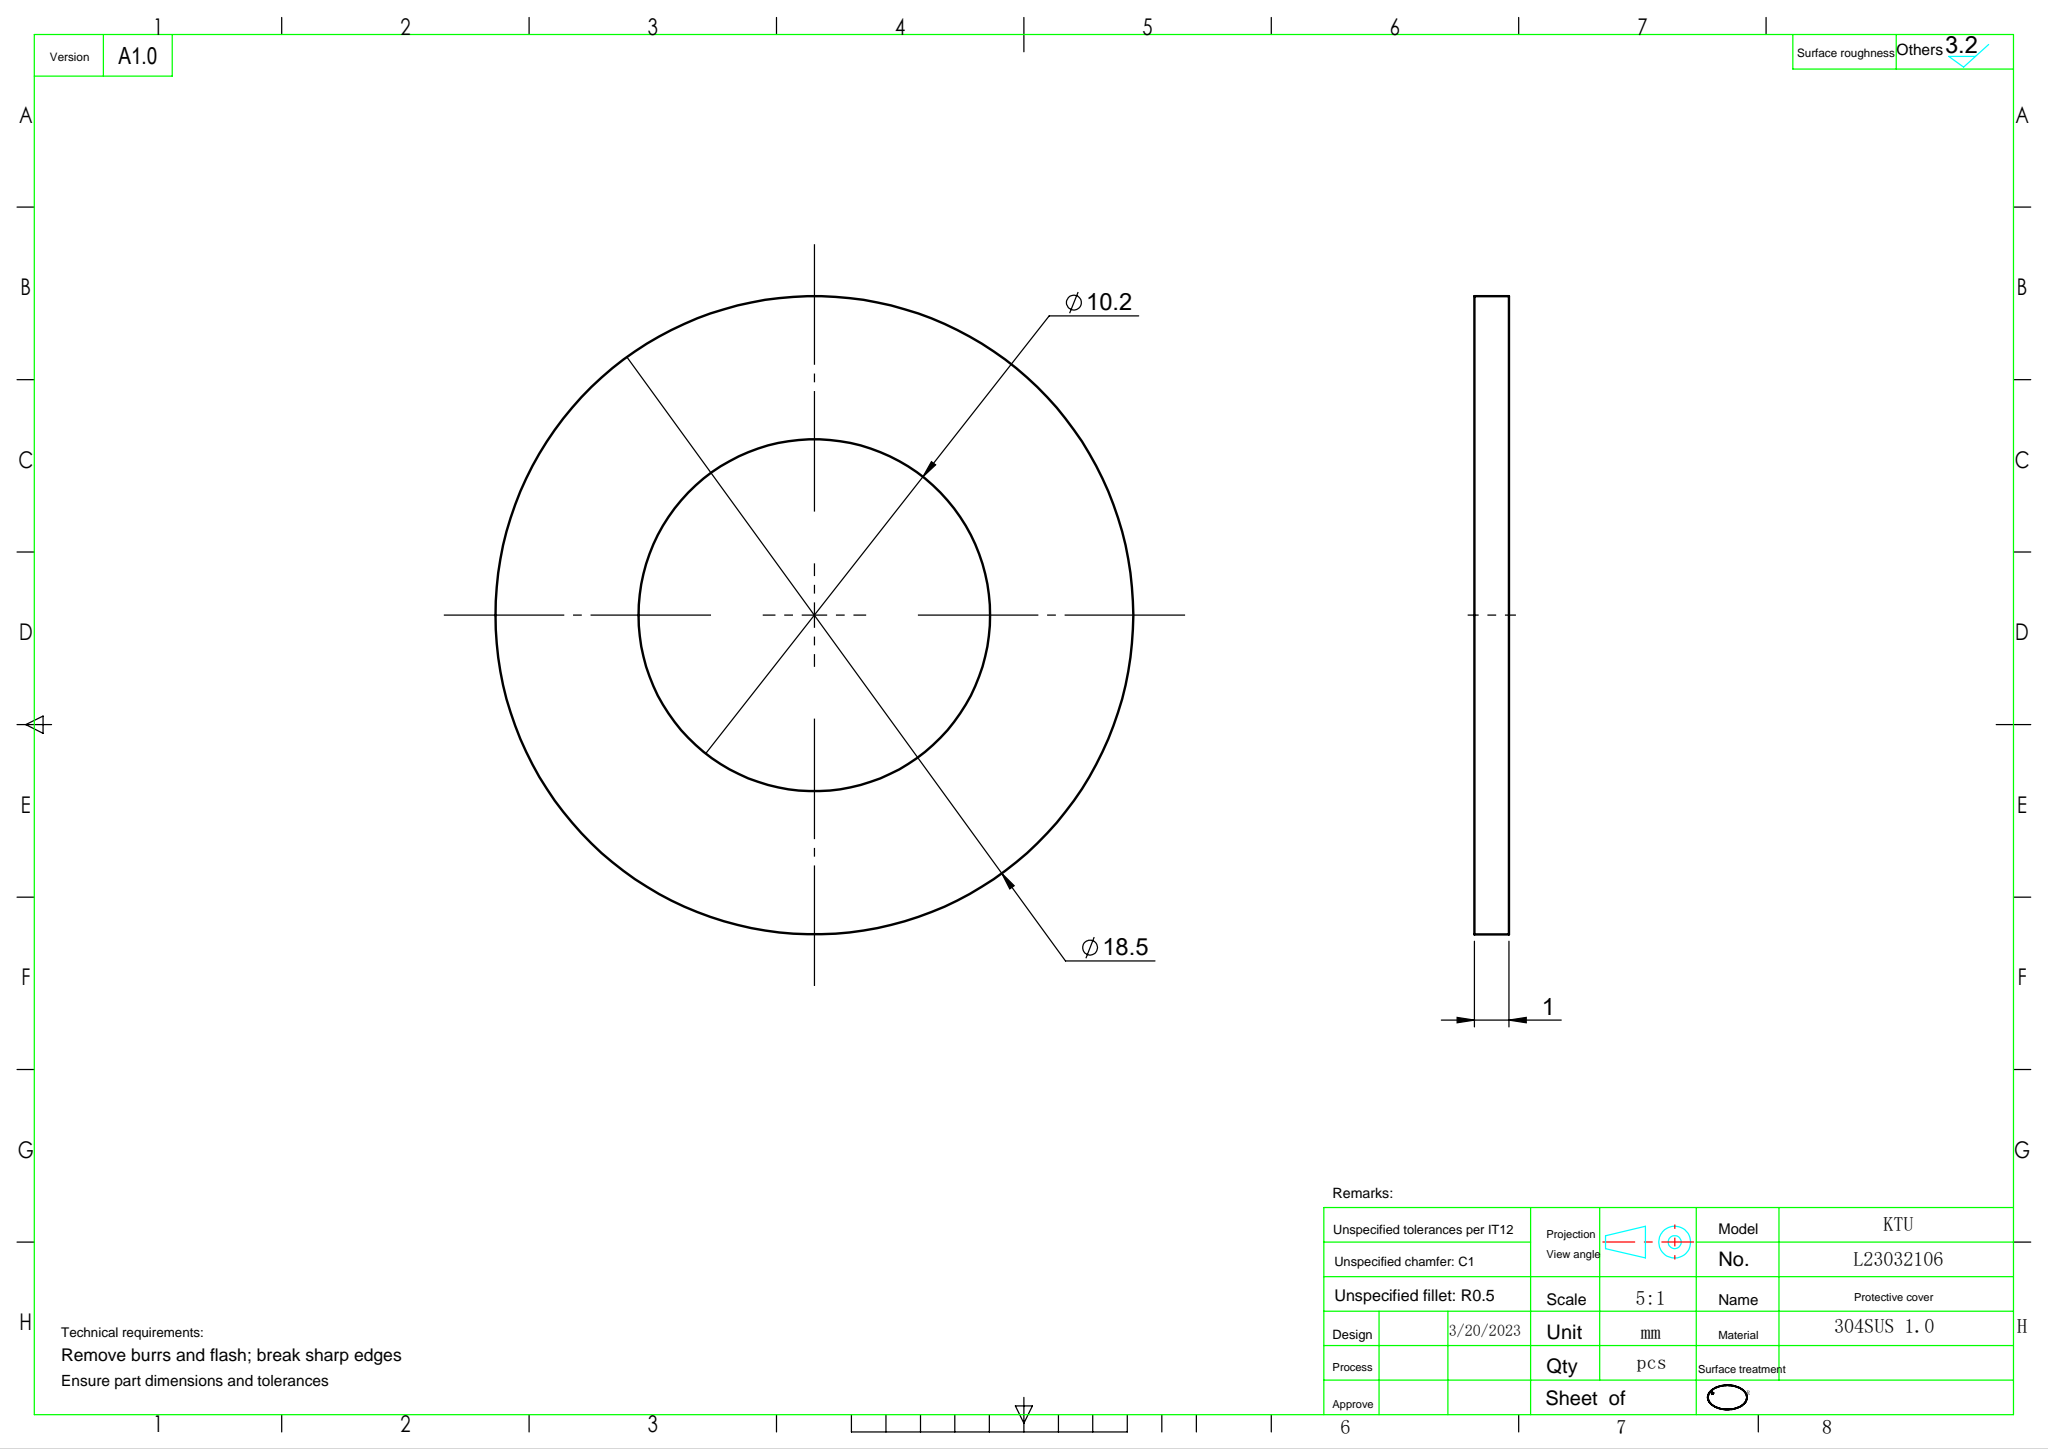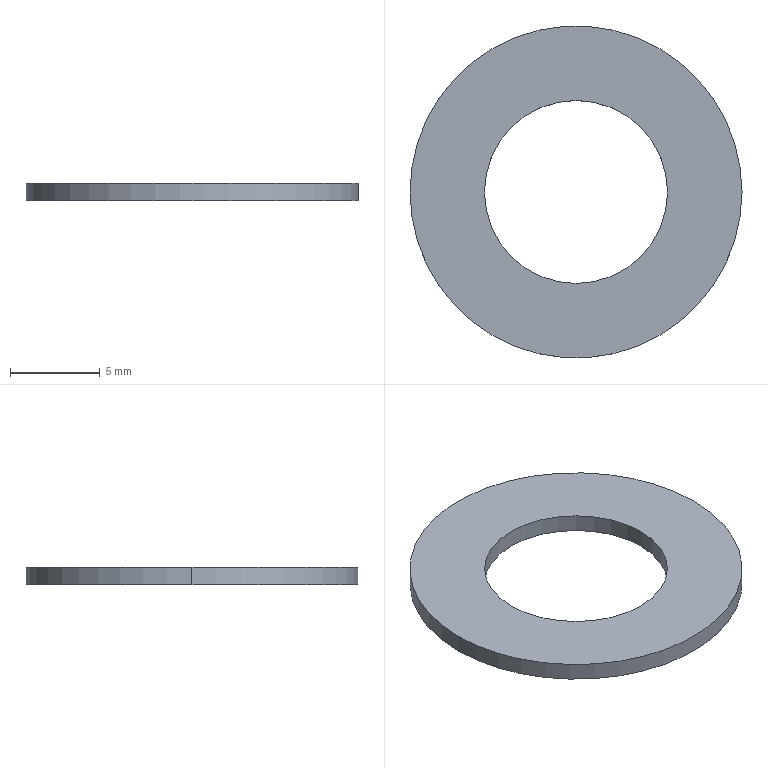Part | SolidWorks | features FlatPattern 1, SMBaseFlange 1, SheetMetal 1 | 1 solid | 6 faces | box 18.5 x 18.5 x 1 mm | volume 187.09 mm3 | cylinder 4 | plane 2 | commonest cylinder face diameters 10.2 x2 18.5 x2
STEP:
#1=CARTESIAN_POINT('',(-5.1,0.,-1.));
#2=VERTEX_POINT('',#1);
#3=CARTESIAN_POINT('',(5.1,0.,-1.));
#4=VERTEX_POINT('',#3);
#5=CARTESIAN_POINT('',(0.,0.,-1.));
#6=DIRECTION('',(0.,0.,1.));
#7=DIRECTION('',(1.,0.,0.));
#8=AXIS2_PLACEMENT_3D('',#5,#6,#7);
#9=CIRCLE('',#8,5.1);
#10=EDGE_CURVE('',#2,#4,#9,.T.);
#11=ORIENTED_EDGE('',*,*,#10,.F.);
#12=CARTESIAN_POINT('',(-5.1,0.,0.));
#13=VERTEX_POINT('',#12);
#14=CARTESIAN_POINT('',(-5.1,0.,-1.));
#15=DIRECTION('',(0.,0.,1.));
#16=VECTOR('',#15,1000.);
#17=LINE('',#14,#16);
#18=EDGE_CURVE('',#2,#13,#17,.T.);
#19=ORIENTED_EDGE('',*,*,#18,.T.);
#20=CARTESIAN_POINT('',(5.1,0.,0.));
#21=VERTEX_POINT('',#20);
#22=CARTESIAN_POINT('',(0.,0.,0.));
#23=DIRECTION('',(0.,0.,1.));
#24=DIRECTION('',(1.,0.,0.));
#25=AXIS2_PLACEMENT_3D('',#22,#23,#24);
#26=CIRCLE('',#25,5.1);
#27=EDGE_CURVE('',#13,#21,#26,.T.);
#28=ORIENTED_EDGE('',*,*,#27,.T.);
#29=CARTESIAN_POINT('',(5.1,0.,-1.));
#30=DIRECTION('',(0.,0.,1.));
#31=VECTOR('',#30,1000.);
#32=LINE('',#29,#31);
#33=EDGE_CURVE('',#4,#21,#32,.T.);
#34=ORIENTED_EDGE('',*,*,#33,.F.);
#35=EDGE_LOOP('',(#11,#19,#28,#34));
#36=FACE_OUTER_BOUND('',#35,.T.);
#37=CARTESIAN_POINT('',(0.,0.,-1.));
#38=DIRECTION('',(0.,0.,1.));
#39=DIRECTION('',(1.,0.,0.));
#40=AXIS2_PLACEMENT_3D('',#37,#38,#39);
#41=CYLINDRICAL_SURFACE('',#40,5.1);
#42=ADVANCED_FACE('',(#36),#41,.F.);
#43=CARTESIAN_POINT('',(9.25,0.,-1.));
#44=VERTEX_POINT('',#43);
#45=CARTESIAN_POINT('',(-9.25,0.,-1.));
#46=VERTEX_POINT('',#45);
#47=CARTESIAN_POINT('',(0.,0.,-1.));
#48=DIRECTION('',(0.,0.,1.));
#49=DIRECTION('',(1.,0.,0.));
#50=AXIS2_PLACEMENT_3D('',#47,#48,#49);
#51=CIRCLE('',#50,9.25);
#52=EDGE_CURVE('',#44,#46,#51,.T.);
#53=ORIENTED_EDGE('',*,*,#52,.T.);
#54=CARTESIAN_POINT('',(-9.25,0.,0.));
#55=VERTEX_POINT('',#54);
#56=CARTESIAN_POINT('',(-9.25,0.,-1.));
#57=DIRECTION('',(0.,0.,1.));
#58=VECTOR('',#57,1000.);
#59=LINE('',#56,#58);
#60=EDGE_CURVE('',#46,#55,#59,.T.);
#61=ORIENTED_EDGE('',*,*,#60,.T.);
#62=CARTESIAN_POINT('',(9.25,0.,0.));
#63=VERTEX_POINT('',#62);
#64=CARTESIAN_POINT('',(0.,0.,0.));
#65=DIRECTION('',(0.,0.,1.));
#66=DIRECTION('',(1.,0.,0.));
#67=AXIS2_PLACEMENT_3D('',#64,#65,#66);
#68=CIRCLE('',#67,9.25);
#69=EDGE_CURVE('',#63,#55,#68,.T.);
#70=ORIENTED_EDGE('',*,*,#69,.F.);
#71=CARTESIAN_POINT('',(9.25,0.,-1.));
#72=DIRECTION('',(0.,0.,1.));
#73=VECTOR('',#72,1000.);
#74=LINE('',#71,#73);
#75=EDGE_CURVE('',#44,#63,#74,.T.);
#76=ORIENTED_EDGE('',*,*,#75,.F.);
#77=EDGE_LOOP('',(#53,#61,#70,#76));
#78=FACE_OUTER_BOUND('',#77,.T.);
#79=CARTESIAN_POINT('',(0.,0.,-1.));
#80=DIRECTION('',(0.,0.,1.));
#81=DIRECTION('',(1.,0.,0.));
#82=AXIS2_PLACEMENT_3D('',#79,#80,#81);
#83=CYLINDRICAL_SURFACE('',#82,9.25);
#84=ADVANCED_FACE('',(#78),#83,.T.);
#85=ORIENTED_EDGE('',*,*,#60,.F.);
#86=CARTESIAN_POINT('',(0.,0.,-1.));
#87=DIRECTION('',(0.,0.,1.));
#88=DIRECTION('',(1.,0.,0.));
#89=AXIS2_PLACEMENT_3D('',#86,#87,#88);
#90=CIRCLE('',#89,9.25);
#91=EDGE_CURVE('',#46,#44,#90,.T.);
#92=ORIENTED_EDGE('',*,*,#91,.T.);
#93=ORIENTED_EDGE('',*,*,#75,.T.);
#94=CARTESIAN_POINT('',(0.,0.,0.));
#95=DIRECTION('',(0.,0.,1.));
#96=DIRECTION('',(1.,0.,0.));
#97=AXIS2_PLACEMENT_3D('',#94,#95,#96);
#98=CIRCLE('',#97,9.25);
#99=EDGE_CURVE('',#55,#63,#98,.T.);
#100=ORIENTED_EDGE('',*,*,#99,.F.);
#101=EDGE_LOOP('',(#85,#92,#93,#100));
#102=FACE_OUTER_BOUND('',#101,.T.);
#103=CARTESIAN_POINT('',(0.,0.,-1.));
#104=DIRECTION('',(0.,0.,1.));
#105=DIRECTION('',(1.,0.,0.));
#106=AXIS2_PLACEMENT_3D('',#103,#104,#105);
#107=CYLINDRICAL_SURFACE('',#106,9.25);
#108=ADVANCED_FACE('',(#102),#107,.T.);
#109=CARTESIAN_POINT('',(0.,0.,-1.));
#110=DIRECTION('',(0.,0.,1.));
#111=DIRECTION('',(1.,0.,0.));
#112=AXIS2_PLACEMENT_3D('',#109,#110,#111);
#113=CIRCLE('',#112,5.1);
#114=EDGE_CURVE('',#4,#2,#113,.T.);
#115=ORIENTED_EDGE('',*,*,#114,.T.);
#116=ORIENTED_EDGE('',*,*,#10,.T.);
#117=EDGE_LOOP('',(#115,#116));
#118=FACE_BOUND('',#117,.T.);
#119=ORIENTED_EDGE('',*,*,#52,.F.);
#120=ORIENTED_EDGE('',*,*,#91,.F.);
#121=EDGE_LOOP('',(#119,#120));
#122=FACE_OUTER_BOUND('',#121,.T.);
#123=CARTESIAN_POINT('',(0.,0.,-1.));
#124=DIRECTION('',(0.,0.,1.));
#125=DIRECTION('',(1.,0.,0.));
#126=AXIS2_PLACEMENT_3D('',#123,#124,#125);
#127=PLANE('',#126);
#128=ADVANCED_FACE('',(#118,#122),#127,.F.);
#129=CARTESIAN_POINT('',(0.,0.,0.));
#130=DIRECTION('',(0.,0.,1.));
#131=DIRECTION('',(1.,0.,0.));
#132=AXIS2_PLACEMENT_3D('',#129,#130,#131);
#133=CIRCLE('',#132,5.1);
#134=EDGE_CURVE('',#21,#13,#133,.T.);
#135=ORIENTED_EDGE('',*,*,#134,.F.);
#136=ORIENTED_EDGE('',*,*,#27,.F.);
#137=EDGE_LOOP('',(#135,#136));
#138=FACE_BOUND('',#137,.T.);
#139=ORIENTED_EDGE('',*,*,#69,.T.);
#140=ORIENTED_EDGE('',*,*,#99,.T.);
#141=EDGE_LOOP('',(#139,#140));
#142=FACE_OUTER_BOUND('',#141,.T.);
#143=CARTESIAN_POINT('',(0.,0.,0.));
#144=DIRECTION('',(0.,0.,1.));
#145=DIRECTION('',(1.,0.,0.));
#146=AXIS2_PLACEMENT_3D('',#143,#144,#145);
#147=PLANE('',#146);
#148=ADVANCED_FACE('',(#138,#142),#147,.T.);
#149=ORIENTED_EDGE('',*,*,#18,.F.);
#150=ORIENTED_EDGE('',*,*,#114,.F.);
#151=ORIENTED_EDGE('',*,*,#33,.T.);
#152=ORIENTED_EDGE('',*,*,#134,.T.);
#153=EDGE_LOOP('',(#149,#150,#151,#152));
#154=FACE_OUTER_BOUND('',#153,.T.);
#155=CARTESIAN_POINT('',(0.,0.,-1.));
#156=DIRECTION('',(0.,0.,1.));
#157=DIRECTION('',(1.,0.,0.));
#158=AXIS2_PLACEMENT_3D('',#155,#156,#157);
#159=CYLINDRICAL_SURFACE('',#158,5.1);
#160=ADVANCED_FACE('',(#154),#159,.F.);
#161=CLOSED_SHELL('',(#42,#84,#108,#128,#148,#160));
#162=MANIFOLD_SOLID_BREP('',#161);
#163=CARTESIAN_POINT('',(0.,0.,0.));
#164=DIRECTION('',(0.,0.,1.));
#165=DIRECTION('',(1.,0.,0.));
#166=AXIS2_PLACEMENT_3D('',#163,#164,#165);
#167=(LENGTH_UNIT()NAMED_UNIT(*)SI_UNIT(.MILLI.,.METRE.));
#168=UNCERTAINTY_MEASURE_WITH_UNIT(LENGTH_MEASURE(0.00001),#167,'','');
#169=(NAMED_UNIT(*)PLANE_ANGLE_UNIT()SI_UNIT($,.RADIAN.));
#170=(NAMED_UNIT(*)SI_UNIT($,.STERADIAN.)SOLID_ANGLE_UNIT());
#171=(GEOMETRIC_REPRESENTATION_CONTEXT(3)GLOBAL_UNCERTAINTY_ASSIGNED_CONTEXT((#168))GLOBAL_UNIT_ASSIGNED_CONTEXT((#167,#169,#170))REPRESENTATION_CONTEXT('',''));
#172=ADVANCED_BREP_SHAPE_REPRESENTATION('',(#162,#166),#171);